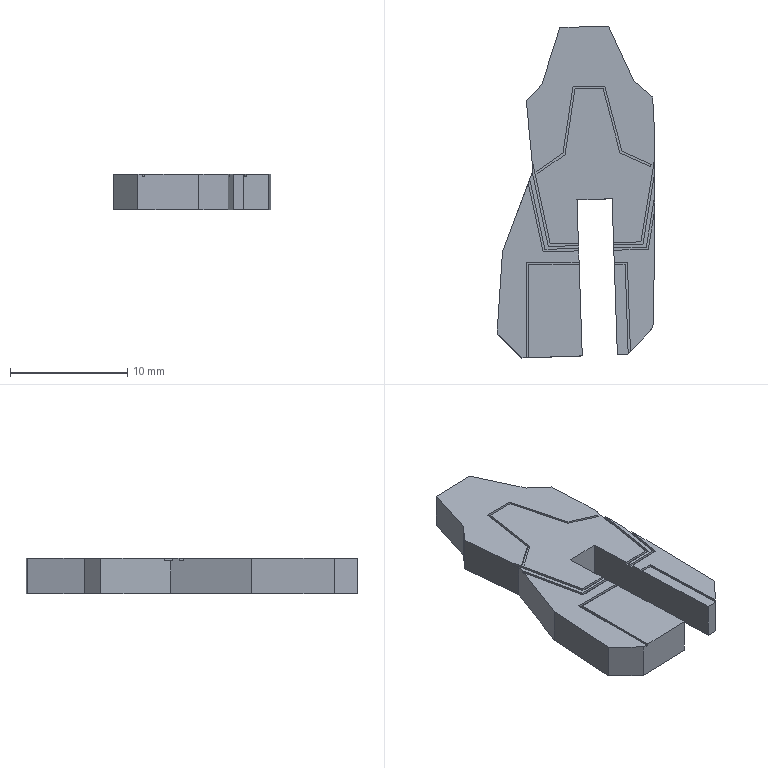Part | SolidWorks | features BaseBody 1 | 1 solid | 72 faces | box 13.49 x 28.35 x 3 mm | volume 780.38 mm3 | plane 58 | spline 14